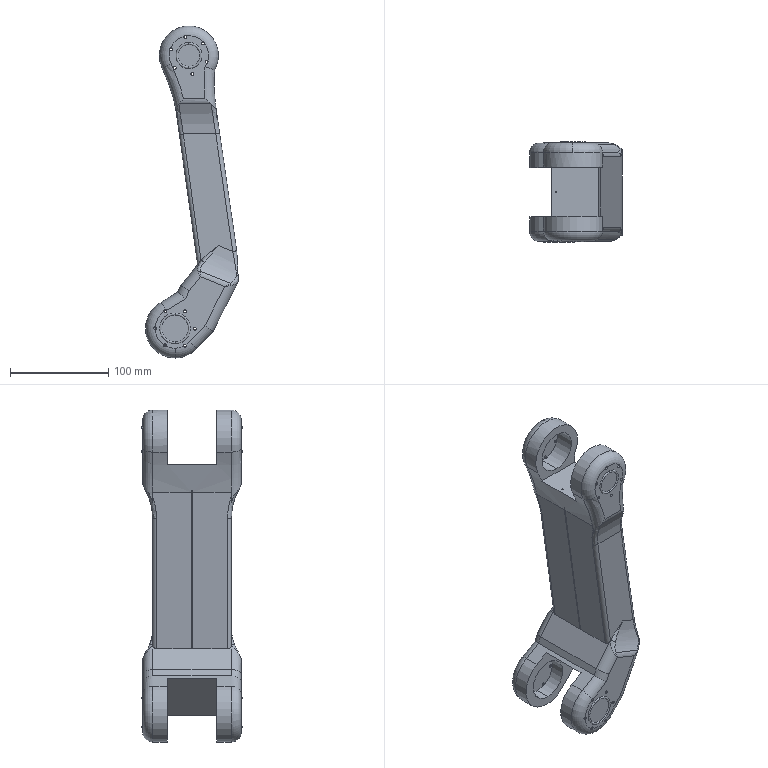Part | SolidWorks | features ICE 10, Fillet 7, CutThin 3, MirrorPattern 3, CirPattern 2, Sweep 2, Extrusion 1 | 1 solid | 170 faces | box 94.476 x 102 x 337.299 mm | volume 1069129 mm3 | cylinder 86 | plane 48 | torus 18 | spline 16 | sphere 2 | commonest cylinder face diameters 3 x48 20 x14 42.4 x8 8 x4 60.144 x4 120 x4